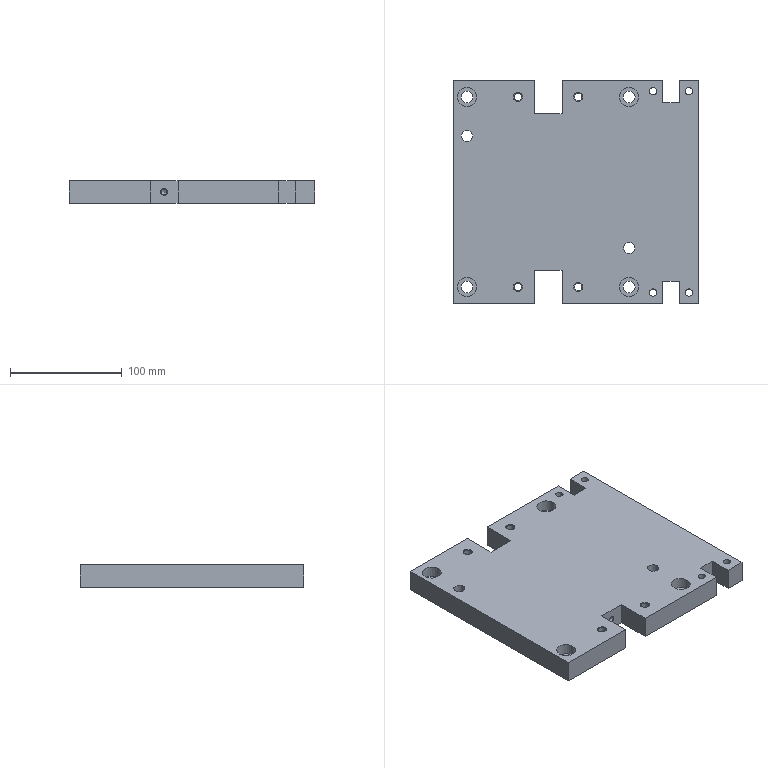Part | STEP file | 冲床-300配套压波_id886_x_t | 1 solid | 66 faces | box 220 x 200 x 20 mm | volume 814165 mm3 | plane 30 | cylinder 24 | cone 12 | commonest cylinder face diameters 6.5 x4 6.8 x4 10.7 x4 11 x4 17 x4 5 x2